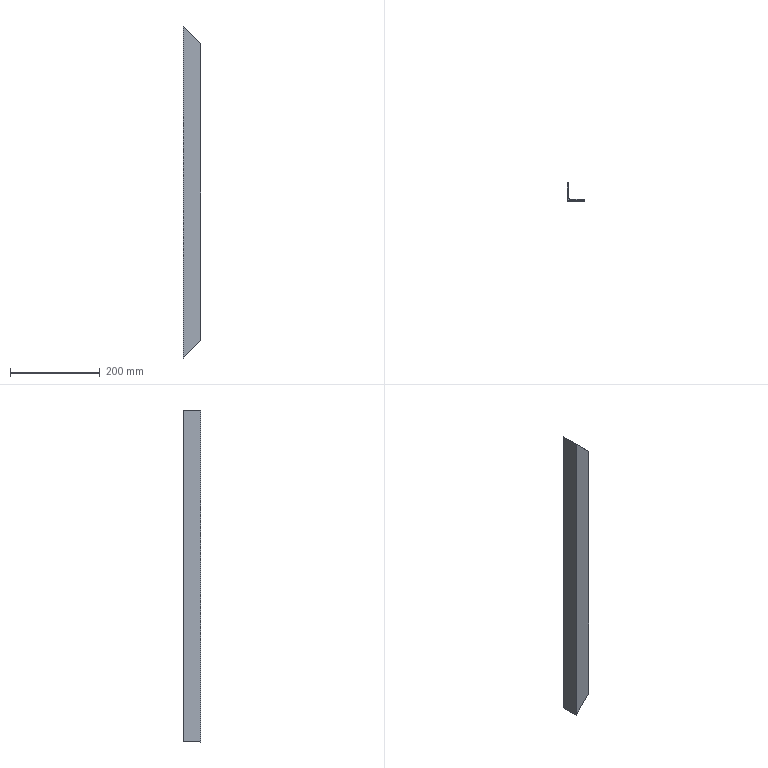Part | SolidWorks | features BaseBody 1 | 1 solid | 11 faces | box 40 x 40 x 740 mm | volume 169434 mm3 | plane 8 | cylinder 3 | commonest cylinder face diameters 2 x2 10 x1
STEP:
#1=CARTESIAN_POINT('',(-10.9,50.9,0.00000005));
#2=VERTEX_POINT('',#1);
#3=CARTESIAN_POINT('',(-10.9,10.9,0.000000025));
#4=VERTEX_POINT('',#3);
#5=CARTESIAN_POINT('',(-10.9,10.9,0.));
#6=DIRECTION('',(0.,-1.,0.));
#7=VECTOR('',#6,1000.);
#8=LINE('',#5,#7);
#9=EDGE_CURVE('',#2,#4,#8,.T.);
#10=ORIENTED_EDGE('',*,*,#9,.T.);
#11=CARTESIAN_POINT('',(-10.9,10.9,740.));
#12=VERTEX_POINT('',#11);
#13=CARTESIAN_POINT('',(-10.9,10.9,0.));
#14=DIRECTION('',(0.,0.,1.));
#15=VECTOR('',#14,1000.);
#16=LINE('',#13,#15);
#17=EDGE_CURVE('',#4,#12,#16,.T.);
#18=ORIENTED_EDGE('',*,*,#17,.T.);
#19=CARTESIAN_POINT('',(-10.9,50.9,740.));
#20=VERTEX_POINT('',#19);
#21=CARTESIAN_POINT('',(-10.9,10.9,740.));
#22=DIRECTION('',(0.,1.,0.));
#23=VECTOR('',#22,1000.);
#24=LINE('',#21,#23);
#25=EDGE_CURVE('',#12,#20,#24,.T.);
#26=ORIENTED_EDGE('',*,*,#25,.T.);
#27=CARTESIAN_POINT('',(-10.9,50.9,0.));
#28=DIRECTION('',(0.,0.,-1.));
#29=VECTOR('',#28,1000.);
#30=LINE('',#27,#29);
#31=EDGE_CURVE('',#20,#2,#30,.T.);
#32=ORIENTED_EDGE('',*,*,#31,.T.);
#33=EDGE_LOOP('',(#10,#18,#26,#32));
#34=FACE_OUTER_BOUND('',#33,.T.);
#35=CARTESIAN_POINT('',(-10.9,10.9,0.));
#36=DIRECTION('',(-1.,0.,0.));
#37=DIRECTION('',(0.,-1.,0.));
#38=AXIS2_PLACEMENT_3D('',#35,#36,#37);
#39=PLANE('',#38);
#40=ADVANCED_FACE('',(#34),#39,.T.);
#41=CARTESIAN_POINT('',(29.1,10.9,40.));
#42=VERTEX_POINT('',#41);
#43=CARTESIAN_POINT('',(-10.9,10.9,0.));
#44=DIRECTION('',(0.7071,0.,0.7071));
#45=VECTOR('',#44,1000.);
#46=LINE('',#43,#45);
#47=EDGE_CURVE('',#4,#42,#46,.T.);
#48=ORIENTED_EDGE('',*,*,#47,.T.);
#49=CARTESIAN_POINT('',(29.1,10.9,700.));
#50=VERTEX_POINT('',#49);
#51=CARTESIAN_POINT('',(29.1,10.9,0.));
#52=DIRECTION('',(0.,0.,1.));
#53=VECTOR('',#52,1000.);
#54=LINE('',#51,#53);
#55=EDGE_CURVE('',#42,#50,#54,.T.);
#56=ORIENTED_EDGE('',*,*,#55,.T.);
#57=CARTESIAN_POINT('',(29.1,10.9,700.));
#58=DIRECTION('',(-0.7071,0.,0.7071));
#59=VECTOR('',#58,1000.);
#60=LINE('',#57,#59);
#61=EDGE_CURVE('',#50,#12,#60,.T.);
#62=ORIENTED_EDGE('',*,*,#61,.T.);
#63=ORIENTED_EDGE('',*,*,#17,.F.);
#64=EDGE_LOOP('',(#48,#56,#62,#63));
#65=FACE_OUTER_BOUND('',#64,.T.);
#66=CARTESIAN_POINT('',(29.1,10.9,0.));
#67=DIRECTION('',(0.,-1.,0.));
#68=DIRECTION('',(1.,0.,0.));
#69=AXIS2_PLACEMENT_3D('',#66,#67,#68);
#70=PLANE('',#69);
#71=ADVANCED_FACE('',(#65),#70,.T.);
#72=CARTESIAN_POINT('',(29.1,12.9,40.));
#73=VERTEX_POINT('',#72);
#74=CARTESIAN_POINT('',(28.1,13.9,39.));
#75=VERTEX_POINT('',#74);
#76=CARTESIAN_POINT('',(29.1,12.9,40.));
#77=CARTESIAN_POINT('',(29.1,13.486,40.));
#78=CARTESIAN_POINT('',(28.686,13.9,39.586));
#79=CARTESIAN_POINT('',(28.1,13.9,39.));
#80=(BOUNDED_CURVE()B_SPLINE_CURVE(3,(#76,#77,#78,#79),.UNSPECIFIED.,.F.,.F.)B_SPLINE_CURVE_WITH_KNOTS((4,4),(0.,1.571),.UNSPECIFIED.)CURVE()GEOMETRIC_REPRESENTATION_ITEM()RATIONAL_B_SPLINE_CURVE((1.,0.8047,0.8047,1.))REPRESENTATION_ITEM(''));
#81=EDGE_CURVE('',#73,#75,#80,.T.);
#82=ORIENTED_EDGE('',*,*,#81,.F.);
#83=CARTESIAN_POINT('',(29.1,0.,40.));
#84=DIRECTION('',(0.,1.,0.));
#85=VECTOR('',#84,1000.);
#86=LINE('',#83,#85);
#87=EDGE_CURVE('',#42,#73,#86,.T.);
#88=ORIENTED_EDGE('',*,*,#87,.F.);
#89=ORIENTED_EDGE('',*,*,#47,.F.);
#90=ORIENTED_EDGE('',*,*,#9,.F.);
#91=CARTESIAN_POINT('',(-8.9,50.9,2.));
#92=VERTEX_POINT('',#91);
#93=CARTESIAN_POINT('',(-5.45,50.9,5.45));
#94=DIRECTION('',(-0.7071,0.,-0.7071));
#95=VECTOR('',#94,1000.);
#96=LINE('',#93,#95);
#97=EDGE_CURVE('',#92,#2,#96,.T.);
#98=ORIENTED_EDGE('',*,*,#97,.F.);
#99=CARTESIAN_POINT('',(-7.9,49.9,3.));
#100=VERTEX_POINT('',#99);
#101=CARTESIAN_POINT('',(-7.9,49.9,3.));
#102=CARTESIAN_POINT('',(-7.9,50.486,3.));
#103=CARTESIAN_POINT('',(-8.314,50.9,2.586));
#104=CARTESIAN_POINT('',(-8.9,50.9,2.));
#105=(BOUNDED_CURVE()B_SPLINE_CURVE(3,(#101,#102,#103,#104),.UNSPECIFIED.,.F.,.F.)B_SPLINE_CURVE_WITH_KNOTS((4,4),(0.,1.571),.UNSPECIFIED.)CURVE()GEOMETRIC_REPRESENTATION_ITEM()RATIONAL_B_SPLINE_CURVE((1.,0.8047,0.8047,1.))REPRESENTATION_ITEM(''));
#106=EDGE_CURVE('',#100,#92,#105,.T.);
#107=ORIENTED_EDGE('',*,*,#106,.F.);
#108=CARTESIAN_POINT('',(-7.9,18.9,3.));
#109=VERTEX_POINT('',#108);
#110=CARTESIAN_POINT('',(-7.9,0.,3.));
#111=DIRECTION('',(0.,1.,0.));
#112=VECTOR('',#111,1000.);
#113=LINE('',#110,#112);
#114=EDGE_CURVE('',#109,#100,#113,.T.);
#115=ORIENTED_EDGE('',*,*,#114,.F.);
#116=CARTESIAN_POINT('',(-2.9,13.9,8.));
#117=VERTEX_POINT('',#116);
#118=CARTESIAN_POINT('',(-2.9,13.9,8.));
#119=CARTESIAN_POINT('',(-5.829,13.9,5.071));
#120=CARTESIAN_POINT('',(-7.9,15.971,3.));
#121=CARTESIAN_POINT('',(-7.9,18.9,3.));
#122=(BOUNDED_CURVE()B_SPLINE_CURVE(3,(#118,#119,#120,#121),.UNSPECIFIED.,.F.,.T.)B_SPLINE_CURVE_WITH_KNOTS((4,4),(1.571,3.142),.UNSPECIFIED.)CURVE()GEOMETRIC_REPRESENTATION_ITEM()RATIONAL_B_SPLINE_CURVE((1.,0.8047,0.8047,1.))REPRESENTATION_ITEM(''));
#123=EDGE_CURVE('',#117,#109,#122,.T.);
#124=ORIENTED_EDGE('',*,*,#123,.F.);
#125=CARTESIAN_POINT('',(-5.45,13.9,5.45));
#126=DIRECTION('',(-0.7071,0.,-0.7071));
#127=VECTOR('',#126,1000.);
#128=LINE('',#125,#127);
#129=EDGE_CURVE('',#75,#117,#128,.T.);
#130=ORIENTED_EDGE('',*,*,#129,.F.);
#131=EDGE_LOOP('',(#82,#88,#89,#90,#98,#107,#115,#124,#130));
#132=FACE_OUTER_BOUND('',#131,.T.);
#133=CARTESIAN_POINT('',(-5.45,0.,5.45));
#134=DIRECTION('',(-0.7071,0.,0.7071));
#135=DIRECTION('',(0.7071,0.,0.7071));
#136=AXIS2_PLACEMENT_3D('',#133,#134,#135);
#137=PLANE('',#136);
#138=ADVANCED_FACE('',(#132),#137,.F.);
#139=ORIENTED_EDGE('',*,*,#97,.T.);
#140=ORIENTED_EDGE('',*,*,#31,.F.);
#141=CARTESIAN_POINT('',(-8.9,50.9,738.));
#142=VERTEX_POINT('',#141);
#143=CARTESIAN_POINT('',(-10.9,50.9,740.));
#144=DIRECTION('',(0.7071,0.,-0.7071));
#145=VECTOR('',#144,1000.);
#146=LINE('',#143,#145);
#147=EDGE_CURVE('',#20,#142,#146,.T.);
#148=ORIENTED_EDGE('',*,*,#147,.T.);
#149=CARTESIAN_POINT('',(-8.9,50.9,0.));
#150=DIRECTION('',(0.,0.,-1.));
#151=VECTOR('',#150,1000.);
#152=LINE('',#149,#151);
#153=EDGE_CURVE('',#142,#92,#152,.T.);
#154=ORIENTED_EDGE('',*,*,#153,.T.);
#155=EDGE_LOOP('',(#139,#140,#148,#154));
#156=FACE_OUTER_BOUND('',#155,.T.);
#157=CARTESIAN_POINT('',(-10.9,50.9,0.));
#158=DIRECTION('',(0.,1.,0.));
#159=DIRECTION('',(-1.,0.,0.));
#160=AXIS2_PLACEMENT_3D('',#157,#158,#159);
#161=PLANE('',#160);
#162=ADVANCED_FACE('',(#156),#161,.T.);
#163=ORIENTED_EDGE('',*,*,#25,.F.);
#164=ORIENTED_EDGE('',*,*,#61,.F.);
#165=CARTESIAN_POINT('',(29.1,12.9,700.));
#166=VERTEX_POINT('',#165);
#167=CARTESIAN_POINT('',(29.1,10.9,700.));
#168=DIRECTION('',(0.,-1.,0.));
#169=VECTOR('',#168,1000.);
#170=LINE('',#167,#169);
#171=EDGE_CURVE('',#166,#50,#170,.T.);
#172=ORIENTED_EDGE('',*,*,#171,.F.);
#173=CARTESIAN_POINT('',(28.1,13.9,701.));
#174=VERTEX_POINT('',#173);
#175=CARTESIAN_POINT('',(28.1,13.9,701.));
#176=CARTESIAN_POINT('',(28.686,13.9,700.414));
#177=CARTESIAN_POINT('',(29.1,13.486,700.));
#178=CARTESIAN_POINT('',(29.1,12.9,700.));
#179=(BOUNDED_CURVE()B_SPLINE_CURVE(3,(#175,#176,#177,#178),.UNSPECIFIED.,.F.,.F.)B_SPLINE_CURVE_WITH_KNOTS((4,4),(1.571,3.142),.UNSPECIFIED.)CURVE()GEOMETRIC_REPRESENTATION_ITEM()RATIONAL_B_SPLINE_CURVE((1.,0.8047,0.8047,1.))REPRESENTATION_ITEM(''));
#180=EDGE_CURVE('',#174,#166,#179,.T.);
#181=ORIENTED_EDGE('',*,*,#180,.F.);
#182=CARTESIAN_POINT('',(-2.9,13.9,732.));
#183=VERTEX_POINT('',#182);
#184=CARTESIAN_POINT('',(29.1,13.9,700.));
#185=DIRECTION('',(0.7071,0.,-0.7071));
#186=VECTOR('',#185,1000.);
#187=LINE('',#184,#186);
#188=EDGE_CURVE('',#183,#174,#187,.T.);
#189=ORIENTED_EDGE('',*,*,#188,.F.);
#190=CARTESIAN_POINT('',(-7.9,18.9,737.));
#191=VERTEX_POINT('',#190);
#192=CARTESIAN_POINT('',(-7.9,18.9,737.));
#193=CARTESIAN_POINT('',(-7.9,15.971,737.));
#194=CARTESIAN_POINT('',(-5.829,13.9,734.929));
#195=CARTESIAN_POINT('',(-2.9,13.9,732.));
#196=(BOUNDED_CURVE()B_SPLINE_CURVE(3,(#192,#193,#194,#195),.UNSPECIFIED.,.F.,.F.)B_SPLINE_CURVE_WITH_KNOTS((4,4),(0.,1.571),.UNSPECIFIED.)CURVE()GEOMETRIC_REPRESENTATION_ITEM()RATIONAL_B_SPLINE_CURVE((1.,0.8047,0.8047,1.))REPRESENTATION_ITEM(''));
#197=EDGE_CURVE('',#191,#183,#196,.T.);
#198=ORIENTED_EDGE('',*,*,#197,.F.);
#199=CARTESIAN_POINT('',(-7.9,49.9,737.));
#200=VERTEX_POINT('',#199);
#201=CARTESIAN_POINT('',(-7.9,10.9,737.));
#202=DIRECTION('',(0.,-1.,0.));
#203=VECTOR('',#202,1000.);
#204=LINE('',#201,#203);
#205=EDGE_CURVE('',#200,#191,#204,.T.);
#206=ORIENTED_EDGE('',*,*,#205,.F.);
#207=CARTESIAN_POINT('',(-8.9,50.9,738.));
#208=CARTESIAN_POINT('',(-8.314,50.9,737.414));
#209=CARTESIAN_POINT('',(-7.9,50.486,737.));
#210=CARTESIAN_POINT('',(-7.9,49.9,737.));
#211=(BOUNDED_CURVE()B_SPLINE_CURVE(3,(#207,#208,#209,#210),.UNSPECIFIED.,.F.,.F.)B_SPLINE_CURVE_WITH_KNOTS((4,4),(1.571,3.142),.UNSPECIFIED.)CURVE()GEOMETRIC_REPRESENTATION_ITEM()RATIONAL_B_SPLINE_CURVE((1.,0.8047,0.8047,1.))REPRESENTATION_ITEM(''));
#212=EDGE_CURVE('',#142,#200,#211,.T.);
#213=ORIENTED_EDGE('',*,*,#212,.F.);
#214=ORIENTED_EDGE('',*,*,#147,.F.);
#215=EDGE_LOOP('',(#163,#164,#172,#181,#189,#198,#206,#213,#214));
#216=FACE_OUTER_BOUND('',#215,.T.);
#217=CARTESIAN_POINT('',(29.1,10.9,700.));
#218=DIRECTION('',(-0.7071,0.,-0.7071));
#219=DIRECTION('',(-0.7071,0.,0.7071));
#220=AXIS2_PLACEMENT_3D('',#217,#218,#219);
#221=PLANE('',#220);
#222=ADVANCED_FACE('',(#216),#221,.F.);
#223=ORIENTED_EDGE('',*,*,#87,.T.);
#224=CARTESIAN_POINT('',(29.1,12.9,0.));
#225=DIRECTION('',(0.,0.,1.));
#226=VECTOR('',#225,1000.);
#227=LINE('',#224,#226);
#228=EDGE_CURVE('',#73,#166,#227,.T.);
#229=ORIENTED_EDGE('',*,*,#228,.T.);
#230=ORIENTED_EDGE('',*,*,#171,.T.);
#231=ORIENTED_EDGE('',*,*,#55,.F.);
#232=EDGE_LOOP('',(#223,#229,#230,#231));
#233=FACE_OUTER_BOUND('',#232,.T.);
#234=CARTESIAN_POINT('',(29.1,12.9,0.));
#235=DIRECTION('',(1.,0.,0.));
#236=DIRECTION('',(0.,1.,0.));
#237=AXIS2_PLACEMENT_3D('',#234,#235,#236);
#238=PLANE('',#237);
#239=ADVANCED_FACE('',(#233),#238,.T.);
#240=ORIENTED_EDGE('',*,*,#129,.T.);
#241=CARTESIAN_POINT('',(-2.9,13.9,0.));
#242=DIRECTION('',(0.,0.,1.));
#243=VECTOR('',#242,1000.);
#244=LINE('',#241,#243);
#245=EDGE_CURVE('',#117,#183,#244,.T.);
#246=ORIENTED_EDGE('',*,*,#245,.T.);
#247=ORIENTED_EDGE('',*,*,#188,.T.);
#248=CARTESIAN_POINT('',(28.1,13.9,0.));
#249=DIRECTION('',(0.,0.,-1.));
#250=VECTOR('',#249,1000.);
#251=LINE('',#248,#250);
#252=EDGE_CURVE('',#174,#75,#251,.T.);
#253=ORIENTED_EDGE('',*,*,#252,.T.);
#254=EDGE_LOOP('',(#240,#246,#247,#253));
#255=FACE_OUTER_BOUND('',#254,.T.);
#256=CARTESIAN_POINT('',(-2.9,13.9,0.));
#257=DIRECTION('',(0.,1.,0.));
#258=DIRECTION('',(-1.,0.,0.));
#259=AXIS2_PLACEMENT_3D('',#256,#257,#258);
#260=PLANE('',#259);
#261=ADVANCED_FACE('',(#255),#260,.T.);
#262=ORIENTED_EDGE('',*,*,#81,.T.);
#263=ORIENTED_EDGE('',*,*,#252,.F.);
#264=ORIENTED_EDGE('',*,*,#180,.T.);
#265=ORIENTED_EDGE('',*,*,#228,.F.);
#266=EDGE_LOOP('',(#262,#263,#264,#265));
#267=FACE_OUTER_BOUND('',#266,.T.);
#268=CARTESIAN_POINT('',(28.1,12.9,0.));
#269=DIRECTION('',(0.,0.,1.));
#270=DIRECTION('',(1.,0.,0.));
#271=AXIS2_PLACEMENT_3D('',#268,#269,#270);
#272=CYLINDRICAL_SURFACE('',#271,1.);
#273=ADVANCED_FACE('',(#267),#272,.T.);
#274=ORIENTED_EDGE('',*,*,#106,.T.);
#275=ORIENTED_EDGE('',*,*,#153,.F.);
#276=ORIENTED_EDGE('',*,*,#212,.T.);
#277=CARTESIAN_POINT('',(-7.9,49.9,0.));
#278=DIRECTION('',(0.,0.,-1.));
#279=VECTOR('',#278,1000.);
#280=LINE('',#277,#279);
#281=EDGE_CURVE('',#200,#100,#280,.T.);
#282=ORIENTED_EDGE('',*,*,#281,.T.);
#283=EDGE_LOOP('',(#274,#275,#276,#282));
#284=FACE_OUTER_BOUND('',#283,.T.);
#285=CARTESIAN_POINT('',(-8.9,49.9,0.));
#286=DIRECTION('',(0.,0.,1.));
#287=DIRECTION('',(1.,0.,0.));
#288=AXIS2_PLACEMENT_3D('',#285,#286,#287);
#289=CYLINDRICAL_SURFACE('',#288,1.);
#290=ADVANCED_FACE('',(#284),#289,.T.);
#291=ORIENTED_EDGE('',*,*,#114,.T.);
#292=ORIENTED_EDGE('',*,*,#281,.F.);
#293=ORIENTED_EDGE('',*,*,#205,.T.);
#294=CARTESIAN_POINT('',(-7.9,18.9,0.));
#295=DIRECTION('',(0.,0.,-1.));
#296=VECTOR('',#295,1000.);
#297=LINE('',#294,#296);
#298=EDGE_CURVE('',#191,#109,#297,.T.);
#299=ORIENTED_EDGE('',*,*,#298,.T.);
#300=EDGE_LOOP('',(#291,#292,#293,#299));
#301=FACE_OUTER_BOUND('',#300,.T.);
#302=CARTESIAN_POINT('',(-7.9,49.9,0.));
#303=DIRECTION('',(1.,0.,0.));
#304=DIRECTION('',(0.,1.,0.));
#305=AXIS2_PLACEMENT_3D('',#302,#303,#304);
#306=PLANE('',#305);
#307=ADVANCED_FACE('',(#301),#306,.T.);
#308=ORIENTED_EDGE('',*,*,#245,.F.);
#309=ORIENTED_EDGE('',*,*,#123,.T.);
#310=ORIENTED_EDGE('',*,*,#298,.F.);
#311=ORIENTED_EDGE('',*,*,#197,.T.);
#312=EDGE_LOOP('',(#308,#309,#310,#311));
#313=FACE_OUTER_BOUND('',#312,.T.);
#314=CARTESIAN_POINT('',(-2.9,18.9,0.));
#315=DIRECTION('',(0.,0.,1.));
#316=DIRECTION('',(1.,0.,0.));
#317=AXIS2_PLACEMENT_3D('',#314,#315,#316);
#318=CYLINDRICAL_SURFACE('',#317,5.);
#319=ADVANCED_FACE('',(#313),#318,.F.);
#320=CLOSED_SHELL('',(#40,#71,#138,#162,#222,#239,#261,#273,#290,#307,#319));
#321=MANIFOLD_SOLID_BREP('',#320);
#322=CARTESIAN_POINT('',(0.,0.,0.));
#323=DIRECTION('',(0.,0.,1.));
#324=DIRECTION('',(1.,0.,0.));
#325=AXIS2_PLACEMENT_3D('',#322,#323,#324);
#326=(LENGTH_UNIT()NAMED_UNIT(*)SI_UNIT(.MILLI.,.METRE.));
#327=UNCERTAINTY_MEASURE_WITH_UNIT(LENGTH_MEASURE(0.00001),#326,'','');
#328=(NAMED_UNIT(*)PLANE_ANGLE_UNIT()SI_UNIT($,.RADIAN.));
#329=(NAMED_UNIT(*)SI_UNIT($,.STERADIAN.)SOLID_ANGLE_UNIT());
#330=(GEOMETRIC_REPRESENTATION_CONTEXT(3)GLOBAL_UNCERTAINTY_ASSIGNED_CONTEXT((#327))GLOBAL_UNIT_ASSIGNED_CONTEXT((#326,#328,#329))REPRESENTATION_CONTEXT('',''));
#331=ADVANCED_BREP_SHAPE_REPRESENTATION('',(#321,#325),#330);